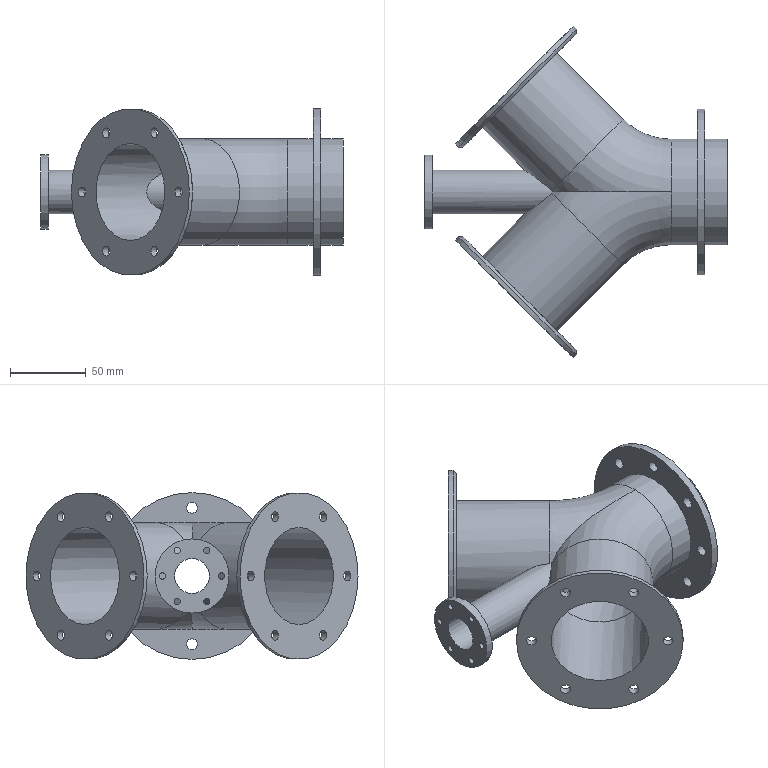Part | STEP file | Pipe Primary Air | 1 solid | 70 faces | box 200 x 219.345 x 110.2 mm | volume 292078 mm3 | cylinder 47 | plane 11 | cone 8 | torus 4 | commonest cylinder face diameters 6.647 x18 7.134 x8 4.134 x6 70.2 x4 64.2 x3 110.2 x3